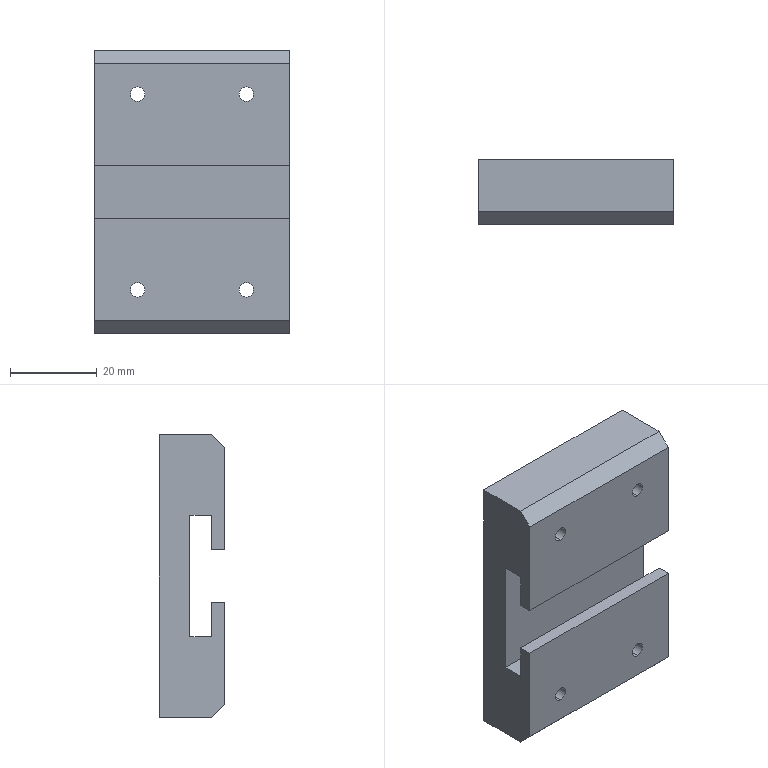Part | SolidWorks | features Chamfer 1, Extrusion 1, HoleWzd 1 | 1 solid | 24 faces | box 45 x 15 x 65 mm | volume 35037 mm3 | plane 16 | cylinder 8 | commonest cylinder face diameters 3.3 x8
STEP:
#1=CARTESIAN_POINT('',(-12.5,-15.,-124.15));
#2=VERTEX_POINT('',#1);
#3=CARTESIAN_POINT('',(-12.5,-15.,-120.85));
#4=VERTEX_POINT('',#3);
#5=CARTESIAN_POINT('',(-12.5,-15.,-122.5));
#6=DIRECTION('',(0.,1.,0.));
#7=DIRECTION('',(0.,0.,1.));
#8=AXIS2_PLACEMENT_3D('',#5,#6,#7);
#9=CIRCLE('',#8,1.65);
#10=EDGE_CURVE('',#2,#4,#9,.T.);
#11=ORIENTED_EDGE('',*,*,#10,.F.);
#12=CARTESIAN_POINT('',(-12.5,0.,-124.15));
#13=VERTEX_POINT('',#12);
#14=CARTESIAN_POINT('',(-12.5,0.,-124.15));
#15=DIRECTION('',(0.,1.,0.));
#16=VECTOR('',#15,1000.);
#17=LINE('',#14,#16);
#18=EDGE_CURVE('',#2,#13,#17,.T.);
#19=ORIENTED_EDGE('',*,*,#18,.T.);
#20=CARTESIAN_POINT('',(-12.5,0.,-120.85));
#21=VERTEX_POINT('',#20);
#22=CARTESIAN_POINT('',(-12.5,0.,-122.5));
#23=DIRECTION('',(0.,1.,0.));
#24=DIRECTION('',(0.,0.,1.));
#25=AXIS2_PLACEMENT_3D('',#22,#23,#24);
#26=CIRCLE('',#25,1.65);
#27=EDGE_CURVE('',#13,#21,#26,.T.);
#28=ORIENTED_EDGE('',*,*,#27,.T.);
#29=CARTESIAN_POINT('',(-12.5,0.,-120.85));
#30=DIRECTION('',(0.,1.,0.));
#31=VECTOR('',#30,1000.);
#32=LINE('',#29,#31);
#33=EDGE_CURVE('',#4,#21,#32,.T.);
#34=ORIENTED_EDGE('',*,*,#33,.F.);
#35=EDGE_LOOP('',(#11,#19,#28,#34));
#36=FACE_OUTER_BOUND('',#35,.T.);
#37=CARTESIAN_POINT('',(-12.5,0.,-122.5));
#38=DIRECTION('',(0.,1.,0.));
#39=DIRECTION('',(0.,0.,1.));
#40=AXIS2_PLACEMENT_3D('',#37,#38,#39);
#41=CYLINDRICAL_SURFACE('',#40,1.65);
#42=ADVANCED_FACE('',(#36),#41,.F.);
#43=CARTESIAN_POINT('',(12.5,-15.,-124.15));
#44=VERTEX_POINT('',#43);
#45=CARTESIAN_POINT('',(12.5,-15.,-120.85));
#46=VERTEX_POINT('',#45);
#47=CARTESIAN_POINT('',(12.5,-15.,-122.5));
#48=DIRECTION('',(0.,1.,0.));
#49=DIRECTION('',(0.,0.,1.));
#50=AXIS2_PLACEMENT_3D('',#47,#48,#49);
#51=CIRCLE('',#50,1.65);
#52=EDGE_CURVE('',#44,#46,#51,.T.);
#53=ORIENTED_EDGE('',*,*,#52,.F.);
#54=CARTESIAN_POINT('',(12.5,0.,-124.15));
#55=VERTEX_POINT('',#54);
#56=CARTESIAN_POINT('',(12.5,0.,-124.15));
#57=DIRECTION('',(0.,1.,0.));
#58=VECTOR('',#57,1000.);
#59=LINE('',#56,#58);
#60=EDGE_CURVE('',#44,#55,#59,.T.);
#61=ORIENTED_EDGE('',*,*,#60,.T.);
#62=CARTESIAN_POINT('',(12.5,0.,-120.85));
#63=VERTEX_POINT('',#62);
#64=CARTESIAN_POINT('',(12.5,0.,-122.5));
#65=DIRECTION('',(0.,1.,0.));
#66=DIRECTION('',(0.,0.,1.));
#67=AXIS2_PLACEMENT_3D('',#64,#65,#66);
#68=CIRCLE('',#67,1.65);
#69=EDGE_CURVE('',#55,#63,#68,.T.);
#70=ORIENTED_EDGE('',*,*,#69,.T.);
#71=CARTESIAN_POINT('',(12.5,0.,-120.85));
#72=DIRECTION('',(0.,1.,0.));
#73=VECTOR('',#72,1000.);
#74=LINE('',#71,#73);
#75=EDGE_CURVE('',#46,#63,#74,.T.);
#76=ORIENTED_EDGE('',*,*,#75,.F.);
#77=EDGE_LOOP('',(#53,#61,#70,#76));
#78=FACE_OUTER_BOUND('',#77,.T.);
#79=CARTESIAN_POINT('',(12.5,0.,-122.5));
#80=DIRECTION('',(0.,1.,0.));
#81=DIRECTION('',(0.,0.,1.));
#82=AXIS2_PLACEMENT_3D('',#79,#80,#81);
#83=CYLINDRICAL_SURFACE('',#82,1.65);
#84=ADVANCED_FACE('',(#78),#83,.F.);
#85=CARTESIAN_POINT('',(-12.5,-15.,-79.15));
#86=VERTEX_POINT('',#85);
#87=CARTESIAN_POINT('',(-12.5,-15.,-75.85));
#88=VERTEX_POINT('',#87);
#89=CARTESIAN_POINT('',(-12.5,-15.,-77.5));
#90=DIRECTION('',(0.,1.,0.));
#91=DIRECTION('',(0.,0.,1.));
#92=AXIS2_PLACEMENT_3D('',#89,#90,#91);
#93=CIRCLE('',#92,1.65);
#94=EDGE_CURVE('',#86,#88,#93,.T.);
#95=ORIENTED_EDGE('',*,*,#94,.F.);
#96=CARTESIAN_POINT('',(-12.5,0.,-79.15));
#97=VERTEX_POINT('',#96);
#98=CARTESIAN_POINT('',(-12.5,0.,-79.15));
#99=DIRECTION('',(0.,1.,0.));
#100=VECTOR('',#99,1000.);
#101=LINE('',#98,#100);
#102=EDGE_CURVE('',#86,#97,#101,.T.);
#103=ORIENTED_EDGE('',*,*,#102,.T.);
#104=CARTESIAN_POINT('',(-12.5,0.,-75.85));
#105=VERTEX_POINT('',#104);
#106=CARTESIAN_POINT('',(-12.5,0.,-77.5));
#107=DIRECTION('',(0.,1.,0.));
#108=DIRECTION('',(0.,0.,1.));
#109=AXIS2_PLACEMENT_3D('',#106,#107,#108);
#110=CIRCLE('',#109,1.65);
#111=EDGE_CURVE('',#97,#105,#110,.T.);
#112=ORIENTED_EDGE('',*,*,#111,.T.);
#113=CARTESIAN_POINT('',(-12.5,0.,-75.85));
#114=DIRECTION('',(0.,1.,0.));
#115=VECTOR('',#114,1000.);
#116=LINE('',#113,#115);
#117=EDGE_CURVE('',#88,#105,#116,.T.);
#118=ORIENTED_EDGE('',*,*,#117,.F.);
#119=EDGE_LOOP('',(#95,#103,#112,#118));
#120=FACE_OUTER_BOUND('',#119,.T.);
#121=CARTESIAN_POINT('',(-12.5,0.,-77.5));
#122=DIRECTION('',(0.,1.,0.));
#123=DIRECTION('',(0.,0.,1.));
#124=AXIS2_PLACEMENT_3D('',#121,#122,#123);
#125=CYLINDRICAL_SURFACE('',#124,1.65);
#126=ADVANCED_FACE('',(#120),#125,.F.);
#127=CARTESIAN_POINT('',(12.5,-15.,-79.15));
#128=VERTEX_POINT('',#127);
#129=CARTESIAN_POINT('',(12.5,-15.,-75.85));
#130=VERTEX_POINT('',#129);
#131=CARTESIAN_POINT('',(12.5,-15.,-77.5));
#132=DIRECTION('',(0.,1.,0.));
#133=DIRECTION('',(0.,0.,1.));
#134=AXIS2_PLACEMENT_3D('',#131,#132,#133);
#135=CIRCLE('',#134,1.65);
#136=EDGE_CURVE('',#128,#130,#135,.T.);
#137=ORIENTED_EDGE('',*,*,#136,.F.);
#138=CARTESIAN_POINT('',(12.5,0.,-79.15));
#139=VERTEX_POINT('',#138);
#140=CARTESIAN_POINT('',(12.5,0.,-79.15));
#141=DIRECTION('',(0.,1.,0.));
#142=VECTOR('',#141,1000.);
#143=LINE('',#140,#142);
#144=EDGE_CURVE('',#128,#139,#143,.T.);
#145=ORIENTED_EDGE('',*,*,#144,.T.);
#146=CARTESIAN_POINT('',(12.5,0.,-75.85));
#147=VERTEX_POINT('',#146);
#148=CARTESIAN_POINT('',(12.5,0.,-77.5));
#149=DIRECTION('',(0.,1.,0.));
#150=DIRECTION('',(0.,0.,1.));
#151=AXIS2_PLACEMENT_3D('',#148,#149,#150);
#152=CIRCLE('',#151,1.65);
#153=EDGE_CURVE('',#139,#147,#152,.T.);
#154=ORIENTED_EDGE('',*,*,#153,.T.);
#155=CARTESIAN_POINT('',(12.5,0.,-75.85));
#156=DIRECTION('',(0.,1.,0.));
#157=VECTOR('',#156,1000.);
#158=LINE('',#155,#157);
#159=EDGE_CURVE('',#130,#147,#158,.T.);
#160=ORIENTED_EDGE('',*,*,#159,.F.);
#161=EDGE_LOOP('',(#137,#145,#154,#160));
#162=FACE_OUTER_BOUND('',#161,.T.);
#163=CARTESIAN_POINT('',(12.5,0.,-77.5));
#164=DIRECTION('',(0.,1.,0.));
#165=DIRECTION('',(0.,0.,1.));
#166=AXIS2_PLACEMENT_3D('',#163,#164,#165);
#167=CYLINDRICAL_SURFACE('',#166,1.65);
#168=ADVANCED_FACE('',(#162),#167,.F.);
#169=CARTESIAN_POINT('',(-12.5,0.,-122.5));
#170=DIRECTION('',(0.,1.,0.));
#171=DIRECTION('',(0.,0.,1.));
#172=AXIS2_PLACEMENT_3D('',#169,#170,#171);
#173=CIRCLE('',#172,1.65);
#174=EDGE_CURVE('',#21,#13,#173,.T.);
#175=ORIENTED_EDGE('',*,*,#174,.F.);
#176=ORIENTED_EDGE('',*,*,#27,.F.);
#177=EDGE_LOOP('',(#175,#176));
#178=FACE_BOUND('',#177,.T.);
#179=CARTESIAN_POINT('',(12.5,0.,-122.5));
#180=DIRECTION('',(0.,1.,0.));
#181=DIRECTION('',(0.,0.,1.));
#182=AXIS2_PLACEMENT_3D('',#179,#180,#181);
#183=CIRCLE('',#182,1.65);
#184=EDGE_CURVE('',#63,#55,#183,.T.);
#185=ORIENTED_EDGE('',*,*,#184,.F.);
#186=ORIENTED_EDGE('',*,*,#69,.F.);
#187=EDGE_LOOP('',(#185,#186));
#188=FACE_BOUND('',#187,.T.);
#189=CARTESIAN_POINT('',(-12.5,0.,-77.5));
#190=DIRECTION('',(0.,1.,0.));
#191=DIRECTION('',(0.,0.,1.));
#192=AXIS2_PLACEMENT_3D('',#189,#190,#191);
#193=CIRCLE('',#192,1.65);
#194=EDGE_CURVE('',#105,#97,#193,.T.);
#195=ORIENTED_EDGE('',*,*,#194,.F.);
#196=ORIENTED_EDGE('',*,*,#111,.F.);
#197=EDGE_LOOP('',(#195,#196));
#198=FACE_BOUND('',#197,.T.);
#199=CARTESIAN_POINT('',(-22.5,0.,-132.5));
#200=VERTEX_POINT('',#199);
#201=CARTESIAN_POINT('',(-22.5,0.,-67.5));
#202=VERTEX_POINT('',#201);
#203=CARTESIAN_POINT('',(-22.5,0.,-67.5));
#204=DIRECTION('',(0.,0.,1.));
#205=VECTOR('',#204,1000.);
#206=LINE('',#203,#205);
#207=EDGE_CURVE('',#200,#202,#206,.T.);
#208=ORIENTED_EDGE('',*,*,#207,.T.);
#209=CARTESIAN_POINT('',(22.5,0.,-67.5));
#210=VERTEX_POINT('',#209);
#211=CARTESIAN_POINT('',(22.5,0.,-67.5));
#212=DIRECTION('',(-1.,0.,0.));
#213=VECTOR('',#212,1000.);
#214=LINE('',#211,#213);
#215=EDGE_CURVE('',#210,#202,#214,.T.);
#216=ORIENTED_EDGE('',*,*,#215,.F.);
#217=CARTESIAN_POINT('',(22.5,0.,-132.5));
#218=VERTEX_POINT('',#217);
#219=CARTESIAN_POINT('',(22.5,0.,-67.5));
#220=DIRECTION('',(0.,0.,1.));
#221=VECTOR('',#220,1000.);
#222=LINE('',#219,#221);
#223=EDGE_CURVE('',#218,#210,#222,.T.);
#224=ORIENTED_EDGE('',*,*,#223,.F.);
#225=CARTESIAN_POINT('',(22.5,0.,-132.5));
#226=DIRECTION('',(-1.,0.,0.));
#227=VECTOR('',#226,1000.);
#228=LINE('',#225,#227);
#229=EDGE_CURVE('',#218,#200,#228,.T.);
#230=ORIENTED_EDGE('',*,*,#229,.T.);
#231=EDGE_LOOP('',(#208,#216,#224,#230));
#232=FACE_OUTER_BOUND('',#231,.T.);
#233=CARTESIAN_POINT('',(12.5,0.,-77.5));
#234=DIRECTION('',(0.,1.,0.));
#235=DIRECTION('',(0.,0.,1.));
#236=AXIS2_PLACEMENT_3D('',#233,#234,#235);
#237=CIRCLE('',#236,1.65);
#238=EDGE_CURVE('',#147,#139,#237,.T.);
#239=ORIENTED_EDGE('',*,*,#238,.F.);
#240=ORIENTED_EDGE('',*,*,#153,.F.);
#241=EDGE_LOOP('',(#239,#240));
#242=FACE_BOUND('',#241,.T.);
#243=CARTESIAN_POINT('',(22.5,0.,-67.5));
#244=DIRECTION('',(0.,-1.,0.));
#245=DIRECTION('',(0.,0.,-1.));
#246=AXIS2_PLACEMENT_3D('',#243,#244,#245);
#247=PLANE('',#246);
#248=ADVANCED_FACE('',(#178,#188,#198,#232,#242),#247,.F.);
#249=CARTESIAN_POINT('',(-22.5,-12.,-67.5));
#250=VERTEX_POINT('',#249);
#251=CARTESIAN_POINT('',(-22.5,0.,-67.5));
#252=DIRECTION('',(0.,-1.,0.));
#253=VECTOR('',#252,1000.);
#254=LINE('',#251,#253);
#255=EDGE_CURVE('',#202,#250,#254,.T.);
#256=ORIENTED_EDGE('',*,*,#255,.T.);
#257=CARTESIAN_POINT('',(22.5,-12.,-67.5));
#258=VERTEX_POINT('',#257);
#259=CARTESIAN_POINT('',(22.5,-12.,-67.5));
#260=DIRECTION('',(1.,0.,0.));
#261=VECTOR('',#260,1000.);
#262=LINE('',#259,#261);
#263=EDGE_CURVE('',#250,#258,#262,.T.);
#264=ORIENTED_EDGE('',*,*,#263,.T.);
#265=CARTESIAN_POINT('',(22.5,0.,-67.5));
#266=DIRECTION('',(0.,-1.,0.));
#267=VECTOR('',#266,1000.);
#268=LINE('',#265,#267);
#269=EDGE_CURVE('',#210,#258,#268,.T.);
#270=ORIENTED_EDGE('',*,*,#269,.F.);
#271=ORIENTED_EDGE('',*,*,#215,.T.);
#272=EDGE_LOOP('',(#256,#264,#270,#271));
#273=FACE_OUTER_BOUND('',#272,.T.);
#274=CARTESIAN_POINT('',(22.5,0.,-67.5));
#275=DIRECTION('',(0.,0.,-1.));
#276=DIRECTION('',(-1.,0.,0.));
#277=AXIS2_PLACEMENT_3D('',#274,#275,#276);
#278=PLANE('',#277);
#279=ADVANCED_FACE('',(#273),#278,.F.);
#280=CARTESIAN_POINT('',(-12.5,-15.,-77.5));
#281=DIRECTION('',(0.,1.,0.));
#282=DIRECTION('',(0.,0.,1.));
#283=AXIS2_PLACEMENT_3D('',#280,#281,#282);
#284=CIRCLE('',#283,1.65);
#285=EDGE_CURVE('',#88,#86,#284,.T.);
#286=ORIENTED_EDGE('',*,*,#285,.T.);
#287=ORIENTED_EDGE('',*,*,#94,.T.);
#288=EDGE_LOOP('',(#286,#287));
#289=FACE_BOUND('',#288,.T.);
#290=CARTESIAN_POINT('',(12.5,-15.,-77.5));
#291=DIRECTION('',(0.,1.,0.));
#292=DIRECTION('',(0.,0.,1.));
#293=AXIS2_PLACEMENT_3D('',#290,#291,#292);
#294=CIRCLE('',#293,1.65);
#295=EDGE_CURVE('',#130,#128,#294,.T.);
#296=ORIENTED_EDGE('',*,*,#295,.T.);
#297=ORIENTED_EDGE('',*,*,#136,.T.);
#298=EDGE_LOOP('',(#296,#297));
#299=FACE_BOUND('',#298,.T.);
#300=CARTESIAN_POINT('',(22.5,-15.,-70.5));
#301=VERTEX_POINT('',#300);
#302=CARTESIAN_POINT('',(22.5,-15.,-94.));
#303=VERTEX_POINT('',#302);
#304=CARTESIAN_POINT('',(22.5,-15.,-67.5));
#305=DIRECTION('',(0.,0.,-1.));
#306=VECTOR('',#305,1000.);
#307=LINE('',#304,#306);
#308=EDGE_CURVE('',#301,#303,#307,.T.);
#309=ORIENTED_EDGE('',*,*,#308,.F.);
#310=CARTESIAN_POINT('',(-22.5,-15.,-70.5));
#311=VERTEX_POINT('',#310);
#312=CARTESIAN_POINT('',(22.5,-15.,-70.5));
#313=DIRECTION('',(-1.,0.,0.));
#314=VECTOR('',#313,1000.);
#315=LINE('',#312,#314);
#316=EDGE_CURVE('',#301,#311,#315,.T.);
#317=ORIENTED_EDGE('',*,*,#316,.T.);
#318=CARTESIAN_POINT('',(-22.5,-15.,-94.));
#319=VERTEX_POINT('',#318);
#320=CARTESIAN_POINT('',(-22.5,-15.,-67.5));
#321=DIRECTION('',(0.,0.,-1.));
#322=VECTOR('',#321,1000.);
#323=LINE('',#320,#322);
#324=EDGE_CURVE('',#311,#319,#323,.T.);
#325=ORIENTED_EDGE('',*,*,#324,.T.);
#326=CARTESIAN_POINT('',(22.5,-15.,-94.));
#327=DIRECTION('',(-1.,0.,0.));
#328=VECTOR('',#327,1000.);
#329=LINE('',#326,#328);
#330=EDGE_CURVE('',#303,#319,#329,.T.);
#331=ORIENTED_EDGE('',*,*,#330,.F.);
#332=EDGE_LOOP('',(#309,#317,#325,#331));
#333=FACE_OUTER_BOUND('',#332,.T.);
#334=CARTESIAN_POINT('',(22.5,-15.,-67.5));
#335=DIRECTION('',(0.,1.,0.));
#336=DIRECTION('',(0.,0.,1.));
#337=AXIS2_PLACEMENT_3D('',#334,#335,#336);
#338=PLANE('',#337);
#339=ADVANCED_FACE('',(#289,#299,#333),#338,.F.);
#340=CARTESIAN_POINT('',(-22.5,-12.,-94.));
#341=VERTEX_POINT('',#340);
#342=CARTESIAN_POINT('',(-22.5,-15.,-94.));
#343=DIRECTION('',(0.,1.,0.));
#344=VECTOR('',#343,1000.);
#345=LINE('',#342,#344);
#346=EDGE_CURVE('',#319,#341,#345,.T.);
#347=ORIENTED_EDGE('',*,*,#346,.T.);
#348=CARTESIAN_POINT('',(22.5,-12.,-94.));
#349=VERTEX_POINT('',#348);
#350=CARTESIAN_POINT('',(22.5,-12.,-94.));
#351=DIRECTION('',(-1.,0.,0.));
#352=VECTOR('',#351,1000.);
#353=LINE('',#350,#352);
#354=EDGE_CURVE('',#349,#341,#353,.T.);
#355=ORIENTED_EDGE('',*,*,#354,.F.);
#356=CARTESIAN_POINT('',(22.5,-15.,-94.));
#357=DIRECTION('',(0.,1.,0.));
#358=VECTOR('',#357,1000.);
#359=LINE('',#356,#358);
#360=EDGE_CURVE('',#303,#349,#359,.T.);
#361=ORIENTED_EDGE('',*,*,#360,.F.);
#362=ORIENTED_EDGE('',*,*,#330,.T.);
#363=EDGE_LOOP('',(#347,#355,#361,#362));
#364=FACE_OUTER_BOUND('',#363,.T.);
#365=CARTESIAN_POINT('',(22.5,-15.,-94.));
#366=DIRECTION('',(0.,0.,1.));
#367=DIRECTION('',(0.,-1.,0.));
#368=AXIS2_PLACEMENT_3D('',#365,#366,#367);
#369=PLANE('',#368);
#370=ADVANCED_FACE('',(#364),#369,.F.);
#371=CARTESIAN_POINT('',(-22.5,-12.,-86.));
#372=VERTEX_POINT('',#371);
#373=CARTESIAN_POINT('',(-22.5,-12.,-94.));
#374=DIRECTION('',(0.,0.,1.));
#375=VECTOR('',#374,1000.);
#376=LINE('',#373,#375);
#377=EDGE_CURVE('',#341,#372,#376,.T.);
#378=ORIENTED_EDGE('',*,*,#377,.T.);
#379=CARTESIAN_POINT('',(22.5,-12.,-86.));
#380=VERTEX_POINT('',#379);
#381=CARTESIAN_POINT('',(22.5,-12.,-86.));
#382=DIRECTION('',(-1.,0.,0.));
#383=VECTOR('',#382,1000.);
#384=LINE('',#381,#383);
#385=EDGE_CURVE('',#380,#372,#384,.T.);
#386=ORIENTED_EDGE('',*,*,#385,.F.);
#387=CARTESIAN_POINT('',(22.5,-12.,-94.));
#388=DIRECTION('',(0.,0.,1.));
#389=VECTOR('',#388,1000.);
#390=LINE('',#387,#389);
#391=EDGE_CURVE('',#349,#380,#390,.T.);
#392=ORIENTED_EDGE('',*,*,#391,.F.);
#393=ORIENTED_EDGE('',*,*,#354,.T.);
#394=EDGE_LOOP('',(#378,#386,#392,#393));
#395=FACE_OUTER_BOUND('',#394,.T.);
#396=CARTESIAN_POINT('',(22.5,-12.,-94.));
#397=DIRECTION('',(0.,-1.,0.));
#398=DIRECTION('',(0.,0.,-1.));
#399=AXIS2_PLACEMENT_3D('',#396,#397,#398);
#400=PLANE('',#399);
#401=ADVANCED_FACE('',(#395),#400,.F.);
#402=CARTESIAN_POINT('',(-22.5,-7.,-86.));
#403=VERTEX_POINT('',#402);
#404=CARTESIAN_POINT('',(-22.5,-12.,-86.));
#405=DIRECTION('',(0.,1.,0.));
#406=VECTOR('',#405,1000.);
#407=LINE('',#404,#406);
#408=EDGE_CURVE('',#372,#403,#407,.T.);
#409=ORIENTED_EDGE('',*,*,#408,.T.);
#410=CARTESIAN_POINT('',(22.5,-7.,-86.));
#411=VERTEX_POINT('',#410);
#412=CARTESIAN_POINT('',(22.5,-7.,-86.));
#413=DIRECTION('',(-1.,0.,0.));
#414=VECTOR('',#413,1000.);
#415=LINE('',#412,#414);
#416=EDGE_CURVE('',#411,#403,#415,.T.);
#417=ORIENTED_EDGE('',*,*,#416,.F.);
#418=CARTESIAN_POINT('',(22.5,-12.,-86.));
#419=DIRECTION('',(0.,1.,0.));
#420=VECTOR('',#419,1000.);
#421=LINE('',#418,#420);
#422=EDGE_CURVE('',#380,#411,#421,.T.);
#423=ORIENTED_EDGE('',*,*,#422,.F.);
#424=ORIENTED_EDGE('',*,*,#385,.T.);
#425=EDGE_LOOP('',(#409,#417,#423,#424));
#426=FACE_OUTER_BOUND('',#425,.T.);
#427=CARTESIAN_POINT('',(22.5,-12.,-86.));
#428=DIRECTION('',(0.,0.,1.));
#429=DIRECTION('',(1.,0.,0.));
#430=AXIS2_PLACEMENT_3D('',#427,#428,#429);
#431=PLANE('',#430);
#432=ADVANCED_FACE('',(#426),#431,.F.);
#433=CARTESIAN_POINT('',(-22.5,-7.,-114.));
#434=VERTEX_POINT('',#433);
#435=CARTESIAN_POINT('',(-22.5,-7.,-86.));
#436=DIRECTION('',(0.,0.,-1.));
#437=VECTOR('',#436,1000.);
#438=LINE('',#435,#437);
#439=EDGE_CURVE('',#403,#434,#438,.T.);
#440=ORIENTED_EDGE('',*,*,#439,.T.);
#441=CARTESIAN_POINT('',(22.5,-7.,-114.));
#442=VERTEX_POINT('',#441);
#443=CARTESIAN_POINT('',(22.5,-7.,-114.));
#444=DIRECTION('',(-1.,0.,0.));
#445=VECTOR('',#444,1000.);
#446=LINE('',#443,#445);
#447=EDGE_CURVE('',#442,#434,#446,.T.);
#448=ORIENTED_EDGE('',*,*,#447,.F.);
#449=CARTESIAN_POINT('',(22.5,-7.,-86.));
#450=DIRECTION('',(0.,0.,-1.));
#451=VECTOR('',#450,1000.);
#452=LINE('',#449,#451);
#453=EDGE_CURVE('',#411,#442,#452,.T.);
#454=ORIENTED_EDGE('',*,*,#453,.F.);
#455=ORIENTED_EDGE('',*,*,#416,.T.);
#456=EDGE_LOOP('',(#440,#448,#454,#455));
#457=FACE_OUTER_BOUND('',#456,.T.);
#458=CARTESIAN_POINT('',(22.5,-7.,-86.));
#459=DIRECTION('',(0.,1.,0.));
#460=DIRECTION('',(0.,0.,1.));
#461=AXIS2_PLACEMENT_3D('',#458,#459,#460);
#462=PLANE('',#461);
#463=ADVANCED_FACE('',(#457),#462,.F.);
#464=CARTESIAN_POINT('',(-22.5,-12.,-114.));
#465=VERTEX_POINT('',#464);
#466=CARTESIAN_POINT('',(-22.5,-12.,-114.));
#467=DIRECTION('',(0.,-1.,0.));
#468=VECTOR('',#467,1000.);
#469=LINE('',#466,#468);
#470=EDGE_CURVE('',#434,#465,#469,.T.);
#471=ORIENTED_EDGE('',*,*,#470,.T.);
#472=CARTESIAN_POINT('',(22.5,-12.,-114.));
#473=VERTEX_POINT('',#472);
#474=CARTESIAN_POINT('',(22.5,-12.,-114.));
#475=DIRECTION('',(-1.,0.,0.));
#476=VECTOR('',#475,1000.);
#477=LINE('',#474,#476);
#478=EDGE_CURVE('',#473,#465,#477,.T.);
#479=ORIENTED_EDGE('',*,*,#478,.F.);
#480=CARTESIAN_POINT('',(22.5,-12.,-114.));
#481=DIRECTION('',(0.,-1.,0.));
#482=VECTOR('',#481,1000.);
#483=LINE('',#480,#482);
#484=EDGE_CURVE('',#442,#473,#483,.T.);
#485=ORIENTED_EDGE('',*,*,#484,.F.);
#486=ORIENTED_EDGE('',*,*,#447,.T.);
#487=EDGE_LOOP('',(#471,#479,#485,#486));
#488=FACE_OUTER_BOUND('',#487,.T.);
#489=CARTESIAN_POINT('',(22.5,-12.,-114.));
#490=DIRECTION('',(0.,0.,-1.));
#491=DIRECTION('',(-1.,0.,0.));
#492=AXIS2_PLACEMENT_3D('',#489,#490,#491);
#493=PLANE('',#492);
#494=ADVANCED_FACE('',(#488),#493,.F.);
#495=CARTESIAN_POINT('',(-22.5,-12.,-106.));
#496=VERTEX_POINT('',#495);
#497=CARTESIAN_POINT('',(-22.5,-12.,-106.));
#498=DIRECTION('',(0.,0.,1.));
#499=VECTOR('',#498,1000.);
#500=LINE('',#497,#499);
#501=EDGE_CURVE('',#465,#496,#500,.T.);
#502=ORIENTED_EDGE('',*,*,#501,.T.);
#503=CARTESIAN_POINT('',(22.5,-12.,-106.));
#504=VERTEX_POINT('',#503);
#505=CARTESIAN_POINT('',(22.5,-12.,-106.));
#506=DIRECTION('',(-1.,0.,0.));
#507=VECTOR('',#506,1000.);
#508=LINE('',#505,#507);
#509=EDGE_CURVE('',#504,#496,#508,.T.);
#510=ORIENTED_EDGE('',*,*,#509,.F.);
#511=CARTESIAN_POINT('',(22.5,-12.,-106.));
#512=DIRECTION('',(0.,0.,1.));
#513=VECTOR('',#512,1000.);
#514=LINE('',#511,#513);
#515=EDGE_CURVE('',#473,#504,#514,.T.);
#516=ORIENTED_EDGE('',*,*,#515,.F.);
#517=ORIENTED_EDGE('',*,*,#478,.T.);
#518=EDGE_LOOP('',(#502,#510,#516,#517));
#519=FACE_OUTER_BOUND('',#518,.T.);
#520=CARTESIAN_POINT('',(22.5,-12.,-106.));
#521=DIRECTION('',(0.,-1.,0.));
#522=DIRECTION('',(0.,0.,-1.));
#523=AXIS2_PLACEMENT_3D('',#520,#521,#522);
#524=PLANE('',#523);
#525=ADVANCED_FACE('',(#519),#524,.F.);
#526=CARTESIAN_POINT('',(-22.5,-15.,-106.));
#527=VERTEX_POINT('',#526);
#528=CARTESIAN_POINT('',(-22.5,-15.,-106.));
#529=DIRECTION('',(0.,-1.,0.));
#530=VECTOR('',#529,1000.);
#531=LINE('',#528,#530);
#532=EDGE_CURVE('',#496,#527,#531,.T.);
#533=ORIENTED_EDGE('',*,*,#532,.T.);
#534=CARTESIAN_POINT('',(22.5,-15.,-106.));
#535=VERTEX_POINT('',#534);
#536=CARTESIAN_POINT('',(22.5,-15.,-106.));
#537=DIRECTION('',(-1.,0.,0.));
#538=VECTOR('',#537,1000.);
#539=LINE('',#536,#538);
#540=EDGE_CURVE('',#535,#527,#539,.T.);
#541=ORIENTED_EDGE('',*,*,#540,.F.);
#542=CARTESIAN_POINT('',(22.5,-15.,-106.));
#543=DIRECTION('',(0.,-1.,0.));
#544=VECTOR('',#543,1000.);
#545=LINE('',#542,#544);
#546=EDGE_CURVE('',#504,#535,#545,.T.);
#547=ORIENTED_EDGE('',*,*,#546,.F.);
#548=ORIENTED_EDGE('',*,*,#509,.T.);
#549=EDGE_LOOP('',(#533,#541,#547,#548));
#550=FACE_OUTER_BOUND('',#549,.T.);
#551=CARTESIAN_POINT('',(22.5,-15.,-106.));
#552=DIRECTION('',(0.,0.,-1.));
#553=DIRECTION('',(0.,1.,0.));
#554=AXIS2_PLACEMENT_3D('',#551,#552,#553);
#555=PLANE('',#554);
#556=ADVANCED_FACE('',(#550),#555,.F.);
#557=CARTESIAN_POINT('',(-12.5,-15.,-122.5));
#558=DIRECTION('',(0.,1.,0.));
#559=DIRECTION('',(0.,0.,1.));
#560=AXIS2_PLACEMENT_3D('',#557,#558,#559);
#561=CIRCLE('',#560,1.65);
#562=EDGE_CURVE('',#4,#2,#561,.T.);
#563=ORIENTED_EDGE('',*,*,#562,.T.);
#564=ORIENTED_EDGE('',*,*,#10,.T.);
#565=EDGE_LOOP('',(#563,#564));
#566=FACE_BOUND('',#565,.T.);
#567=CARTESIAN_POINT('',(12.5,-15.,-122.5));
#568=DIRECTION('',(0.,1.,0.));
#569=DIRECTION('',(0.,0.,1.));
#570=AXIS2_PLACEMENT_3D('',#567,#568,#569);
#571=CIRCLE('',#570,1.65);
#572=EDGE_CURVE('',#46,#44,#571,.T.);
#573=ORIENTED_EDGE('',*,*,#572,.T.);
#574=ORIENTED_EDGE('',*,*,#52,.T.);
#575=EDGE_LOOP('',(#573,#574));
#576=FACE_BOUND('',#575,.T.);
#577=CARTESIAN_POINT('',(-22.5,-15.,-129.5));
#578=VERTEX_POINT('',#577);
#579=CARTESIAN_POINT('',(-22.5,-15.,-106.));
#580=DIRECTION('',(0.,0.,-1.));
#581=VECTOR('',#580,1000.);
#582=LINE('',#579,#581);
#583=EDGE_CURVE('',#527,#578,#582,.T.);
#584=ORIENTED_EDGE('',*,*,#583,.T.);
#585=CARTESIAN_POINT('',(22.5,-15.,-129.5));
#586=VERTEX_POINT('',#585);
#587=CARTESIAN_POINT('',(22.5,-15.,-129.5));
#588=DIRECTION('',(1.,0.,0.));
#589=VECTOR('',#588,1000.);
#590=LINE('',#587,#589);
#591=EDGE_CURVE('',#578,#586,#590,.T.);
#592=ORIENTED_EDGE('',*,*,#591,.T.);
#593=CARTESIAN_POINT('',(22.5,-15.,-106.));
#594=DIRECTION('',(0.,0.,-1.));
#595=VECTOR('',#594,1000.);
#596=LINE('',#593,#595);
#597=EDGE_CURVE('',#535,#586,#596,.T.);
#598=ORIENTED_EDGE('',*,*,#597,.F.);
#599=ORIENTED_EDGE('',*,*,#540,.T.);
#600=EDGE_LOOP('',(#584,#592,#598,#599));
#601=FACE_OUTER_BOUND('',#600,.T.);
#602=CARTESIAN_POINT('',(22.5,-15.,-106.));
#603=DIRECTION('',(0.,1.,0.));
#604=DIRECTION('',(0.,0.,1.));
#605=AXIS2_PLACEMENT_3D('',#602,#603,#604);
#606=PLANE('',#605);
#607=ADVANCED_FACE('',(#566,#576,#601),#606,.F.);
#608=CARTESIAN_POINT('',(22.5,-12.,-132.5));
#609=VERTEX_POINT('',#608);
#610=CARTESIAN_POINT('',(22.5,0.,-132.5));
#611=DIRECTION('',(0.,1.,0.));
#612=VECTOR('',#611,1000.);
#613=LINE('',#610,#612);
#614=EDGE_CURVE('',#609,#218,#613,.T.);
#615=ORIENTED_EDGE('',*,*,#614,.F.);
#616=CARTESIAN_POINT('',(-22.5,-12.,-132.5));
#617=VERTEX_POINT('',#616);
#618=CARTESIAN_POINT('',(22.5,-12.,-132.5));
#619=DIRECTION('',(-1.,0.,0.));
#620=VECTOR('',#619,1000.);
#621=LINE('',#618,#620);
#622=EDGE_CURVE('',#609,#617,#621,.T.);
#623=ORIENTED_EDGE('',*,*,#622,.T.);
#624=CARTESIAN_POINT('',(-22.5,0.,-132.5));
#625=DIRECTION('',(0.,1.,0.));
#626=VECTOR('',#625,1000.);
#627=LINE('',#624,#626);
#628=EDGE_CURVE('',#617,#200,#627,.T.);
#629=ORIENTED_EDGE('',*,*,#628,.T.);
#630=ORIENTED_EDGE('',*,*,#229,.F.);
#631=EDGE_LOOP('',(#615,#623,#629,#630));
#632=FACE_OUTER_BOUND('',#631,.T.);
#633=CARTESIAN_POINT('',(22.5,0.,-132.5));
#634=DIRECTION('',(0.,0.,1.));
#635=DIRECTION('',(0.,-1.,0.));
#636=AXIS2_PLACEMENT_3D('',#633,#634,#635);
#637=PLANE('',#636);
#638=ADVANCED_FACE('',(#632),#637,.F.);
#639=ORIENTED_EDGE('',*,*,#597,.T.);
#640=CARTESIAN_POINT('',(22.5,-72.25,-72.25));
#641=DIRECTION('',(0.,0.7071,-0.7071));
#642=VECTOR('',#641,1000.);
#643=LINE('',#640,#642);
#644=EDGE_CURVE('',#586,#609,#643,.T.);
#645=ORIENTED_EDGE('',*,*,#644,.T.);
#646=ORIENTED_EDGE('',*,*,#614,.T.);
#647=ORIENTED_EDGE('',*,*,#223,.T.);
#648=ORIENTED_EDGE('',*,*,#269,.T.);
#649=CARTESIAN_POINT('',(22.5,27.75,-27.75));
#650=DIRECTION('',(0.,-0.7071,-0.7071));
#651=VECTOR('',#650,1000.);
#652=LINE('',#649,#651);
#653=EDGE_CURVE('',#258,#301,#652,.T.);
#654=ORIENTED_EDGE('',*,*,#653,.T.);
#655=ORIENTED_EDGE('',*,*,#308,.T.);
#656=ORIENTED_EDGE('',*,*,#360,.T.);
#657=ORIENTED_EDGE('',*,*,#391,.T.);
#658=ORIENTED_EDGE('',*,*,#422,.T.);
#659=ORIENTED_EDGE('',*,*,#453,.T.);
#660=ORIENTED_EDGE('',*,*,#484,.T.);
#661=ORIENTED_EDGE('',*,*,#515,.T.);
#662=ORIENTED_EDGE('',*,*,#546,.T.);
#663=EDGE_LOOP('',(#639,#645,#646,#647,#648,#654,#655,#656,#657,#658,#659,#660,#661,#662));
#664=FACE_OUTER_BOUND('',#663,.T.);
#665=CARTESIAN_POINT('',(22.5,0.,0.));
#666=DIRECTION('',(1.,0.,0.));
#667=DIRECTION('',(0.,0.,-1.));
#668=AXIS2_PLACEMENT_3D('',#665,#666,#667);
#669=PLANE('',#668);
#670=ADVANCED_FACE('',(#664),#669,.T.);
#671=ORIENTED_EDGE('',*,*,#628,.F.);
#672=CARTESIAN_POINT('',(-22.5,-12.,-132.5));
#673=DIRECTION('',(0.,-0.7071,0.7071));
#674=VECTOR('',#673,1000.);
#675=LINE('',#672,#674);
#676=EDGE_CURVE('',#617,#578,#675,.T.);
#677=ORIENTED_EDGE('',*,*,#676,.T.);
#678=ORIENTED_EDGE('',*,*,#583,.F.);
#679=ORIENTED_EDGE('',*,*,#532,.F.);
#680=ORIENTED_EDGE('',*,*,#501,.F.);
#681=ORIENTED_EDGE('',*,*,#470,.F.);
#682=ORIENTED_EDGE('',*,*,#439,.F.);
#683=ORIENTED_EDGE('',*,*,#408,.F.);
#684=ORIENTED_EDGE('',*,*,#377,.F.);
#685=ORIENTED_EDGE('',*,*,#346,.F.);
#686=ORIENTED_EDGE('',*,*,#324,.F.);
#687=CARTESIAN_POINT('',(-22.5,-15.,-70.5));
#688=DIRECTION('',(0.,0.7071,0.7071));
#689=VECTOR('',#688,1000.);
#690=LINE('',#687,#689);
#691=EDGE_CURVE('',#311,#250,#690,.T.);
#692=ORIENTED_EDGE('',*,*,#691,.T.);
#693=ORIENTED_EDGE('',*,*,#255,.F.);
#694=ORIENTED_EDGE('',*,*,#207,.F.);
#695=EDGE_LOOP('',(#671,#677,#678,#679,#680,#681,#682,#683,#684,#685,#686,#692,#693,#694));
#696=FACE_OUTER_BOUND('',#695,.T.);
#697=CARTESIAN_POINT('',(-22.5,0.,0.));
#698=DIRECTION('',(1.,0.,0.));
#699=DIRECTION('',(0.,0.,-1.));
#700=AXIS2_PLACEMENT_3D('',#697,#698,#699);
#701=PLANE('',#700);
#702=ADVANCED_FACE('',(#696),#701,.F.);
#703=ORIENTED_EDGE('',*,*,#644,.F.);
#704=ORIENTED_EDGE('',*,*,#591,.F.);
#705=ORIENTED_EDGE('',*,*,#676,.F.);
#706=ORIENTED_EDGE('',*,*,#622,.F.);
#707=EDGE_LOOP('',(#703,#704,#705,#706));
#708=FACE_OUTER_BOUND('',#707,.T.);
#709=CARTESIAN_POINT('',(22.5,-12.,-132.5));
#710=DIRECTION('',(0.,0.7071,0.7071));
#711=DIRECTION('',(-1.,0.,0.));
#712=AXIS2_PLACEMENT_3D('',#709,#710,#711);
#713=PLANE('',#712);
#714=ADVANCED_FACE('',(#708),#713,.F.);
#715=ORIENTED_EDGE('',*,*,#653,.F.);
#716=ORIENTED_EDGE('',*,*,#263,.F.);
#717=ORIENTED_EDGE('',*,*,#691,.F.);
#718=ORIENTED_EDGE('',*,*,#316,.F.);
#719=EDGE_LOOP('',(#715,#716,#717,#718));
#720=FACE_OUTER_BOUND('',#719,.T.);
#721=CARTESIAN_POINT('',(22.5,-15.,-70.5));
#722=DIRECTION('',(0.,0.7071,-0.7071));
#723=DIRECTION('',(-1.,0.,0.));
#724=AXIS2_PLACEMENT_3D('',#721,#722,#723);
#725=PLANE('',#724);
#726=ADVANCED_FACE('',(#720),#725,.F.);
#727=ORIENTED_EDGE('',*,*,#144,.F.);
#728=ORIENTED_EDGE('',*,*,#295,.F.);
#729=ORIENTED_EDGE('',*,*,#159,.T.);
#730=ORIENTED_EDGE('',*,*,#238,.T.);
#731=EDGE_LOOP('',(#727,#728,#729,#730));
#732=FACE_OUTER_BOUND('',#731,.T.);
#733=CARTESIAN_POINT('',(12.5,0.,-77.5));
#734=DIRECTION('',(0.,1.,0.));
#735=DIRECTION('',(0.,0.,1.));
#736=AXIS2_PLACEMENT_3D('',#733,#734,#735);
#737=CYLINDRICAL_SURFACE('',#736,1.65);
#738=ADVANCED_FACE('',(#732),#737,.F.);
#739=ORIENTED_EDGE('',*,*,#102,.F.);
#740=ORIENTED_EDGE('',*,*,#285,.F.);
#741=ORIENTED_EDGE('',*,*,#117,.T.);
#742=ORIENTED_EDGE('',*,*,#194,.T.);
#743=EDGE_LOOP('',(#739,#740,#741,#742));
#744=FACE_OUTER_BOUND('',#743,.T.);
#745=CARTESIAN_POINT('',(-12.5,0.,-77.5));
#746=DIRECTION('',(0.,1.,0.));
#747=DIRECTION('',(0.,0.,1.));
#748=AXIS2_PLACEMENT_3D('',#745,#746,#747);
#749=CYLINDRICAL_SURFACE('',#748,1.65);
#750=ADVANCED_FACE('',(#744),#749,.F.);
#751=ORIENTED_EDGE('',*,*,#60,.F.);
#752=ORIENTED_EDGE('',*,*,#572,.F.);
#753=ORIENTED_EDGE('',*,*,#75,.T.);
#754=ORIENTED_EDGE('',*,*,#184,.T.);
#755=EDGE_LOOP('',(#751,#752,#753,#754));
#756=FACE_OUTER_BOUND('',#755,.T.);
#757=CARTESIAN_POINT('',(12.5,0.,-122.5));
#758=DIRECTION('',(0.,1.,0.));
#759=DIRECTION('',(0.,0.,1.));
#760=AXIS2_PLACEMENT_3D('',#757,#758,#759);
#761=CYLINDRICAL_SURFACE('',#760,1.65);
#762=ADVANCED_FACE('',(#756),#761,.F.);
#763=ORIENTED_EDGE('',*,*,#18,.F.);
#764=ORIENTED_EDGE('',*,*,#562,.F.);
#765=ORIENTED_EDGE('',*,*,#33,.T.);
#766=ORIENTED_EDGE('',*,*,#174,.T.);
#767=EDGE_LOOP('',(#763,#764,#765,#766));
#768=FACE_OUTER_BOUND('',#767,.T.);
#769=CARTESIAN_POINT('',(-12.5,0.,-122.5));
#770=DIRECTION('',(0.,1.,0.));
#771=DIRECTION('',(0.,0.,1.));
#772=AXIS2_PLACEMENT_3D('',#769,#770,#771);
#773=CYLINDRICAL_SURFACE('',#772,1.65);
#774=ADVANCED_FACE('',(#768),#773,.F.);
#775=CLOSED_SHELL('',(#42,#84,#126,#168,#248,#279,#339,#370,#401,#432,#463,#494,#525,#556,#607,#638,#670,#702,#714,#726,#738,#750,#762,#774));
#776=MANIFOLD_SOLID_BREP('',#775);
#777=CARTESIAN_POINT('',(0.,0.,0.));
#778=DIRECTION('',(0.,0.,1.));
#779=DIRECTION('',(1.,0.,0.));
#780=AXIS2_PLACEMENT_3D('',#777,#778,#779);
#781=(LENGTH_UNIT()NAMED_UNIT(*)SI_UNIT(.MILLI.,.METRE.));
#782=UNCERTAINTY_MEASURE_WITH_UNIT(LENGTH_MEASURE(0.00001),#781,'','');
#783=(NAMED_UNIT(*)PLANE_ANGLE_UNIT()SI_UNIT($,.RADIAN.));
#784=(NAMED_UNIT(*)SI_UNIT($,.STERADIAN.)SOLID_ANGLE_UNIT());
#785=(GEOMETRIC_REPRESENTATION_CONTEXT(3)GLOBAL_UNCERTAINTY_ASSIGNED_CONTEXT((#782))GLOBAL_UNIT_ASSIGNED_CONTEXT((#781,#783,#784))REPRESENTATION_CONTEXT('',''));
#786=ADVANCED_BREP_SHAPE_REPRESENTATION('',(#776,#780),#785);